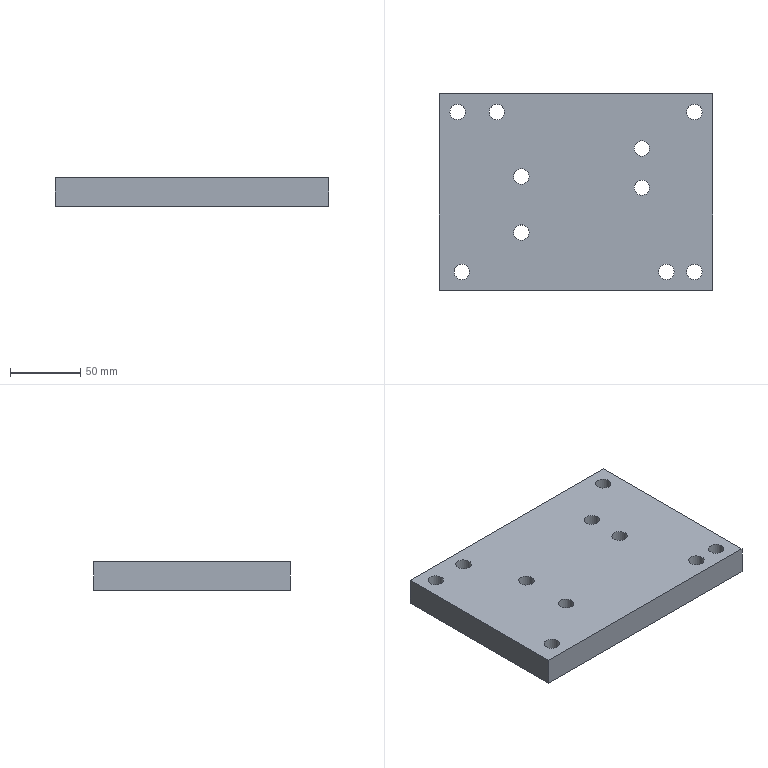Part | STEP file | 110_id2910_x_t | 1 solid | 16 faces | box 195 x 140 x 20 mm | volume 526993 mm3 | cylinder 10 | plane 6 | commonest cylinder face diameters 11 x10